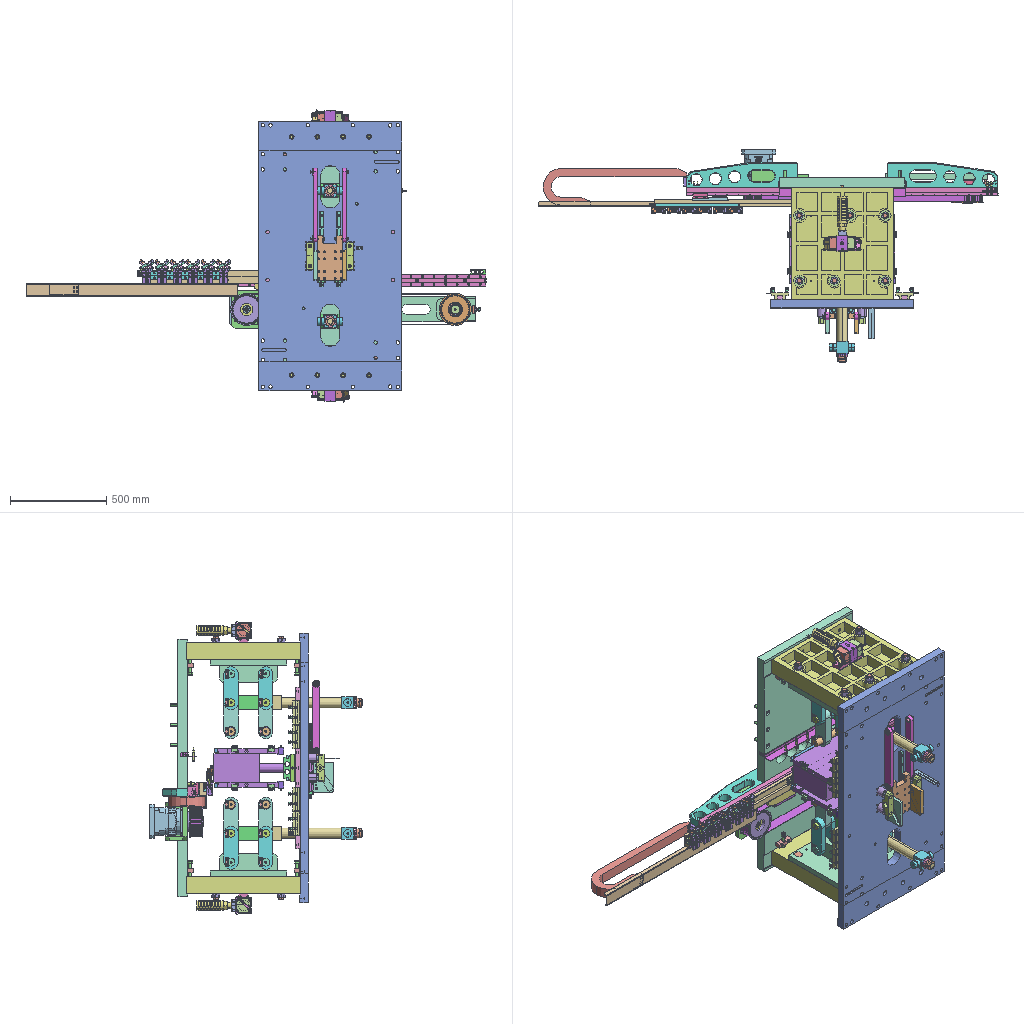Assembly | STEP file | 127 different items | 785 placed | box 2393 x 1108 x 1521 mm
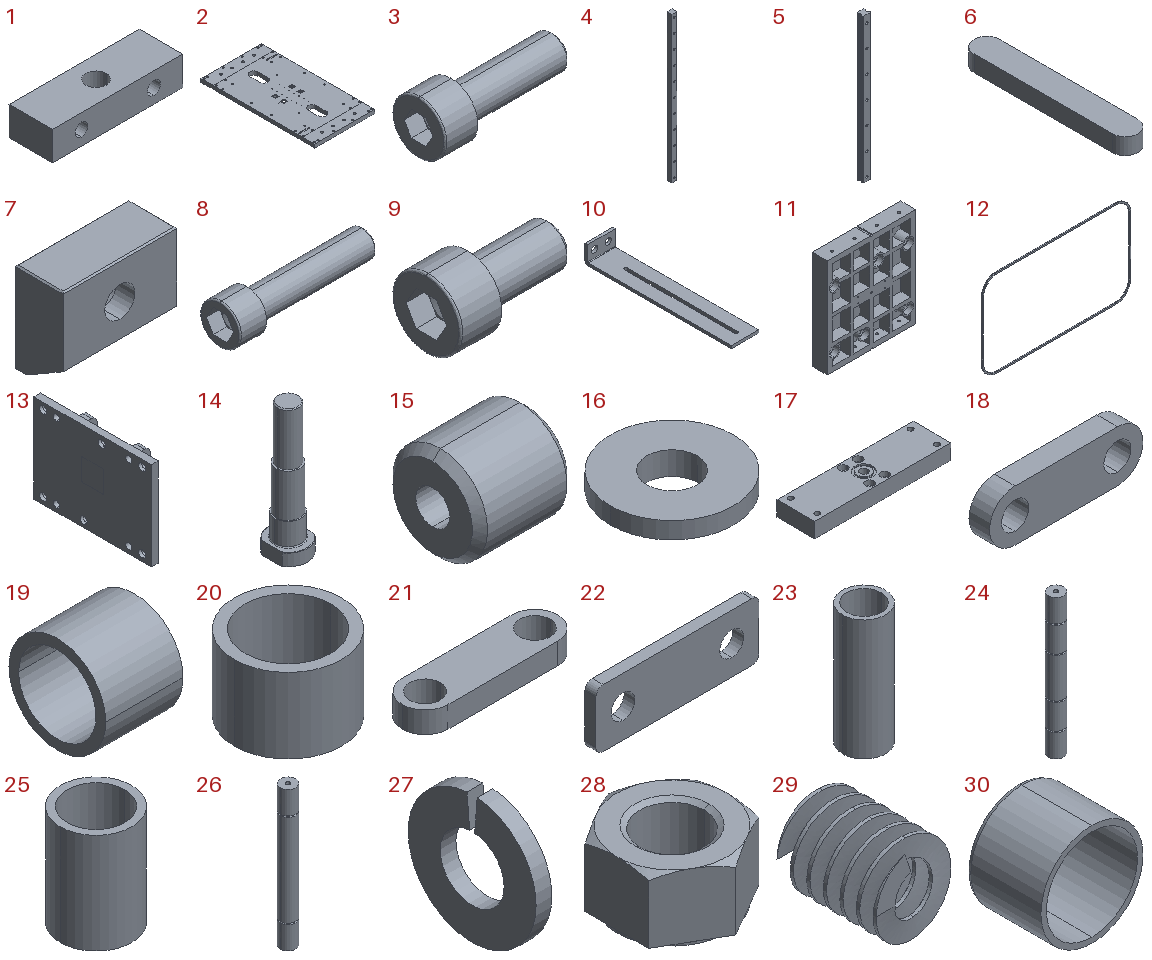Parts list (item | name | quantity | parent item | size | volume):
1 | M-05-2507_default | x8 | in LM06S-05-03-02B_default, LM06S-05-02-04 modified_default | 90 x 30 x 20 mm | 45159 mm3
2 | LM-05-1222B_default | x1 | in LM06S-05-03-02B_default | 742 x 1400 x 44 mm | 38795676 mm3
3 | PN_0075_default | x22 | in LM06S-05-03-02B_default | 33 x 13 x 13 mm | 2167 mm3
4 | P-008160^LM06S-05-03-02B_default | x2 | in LM06S-05-03-02B_default | 28 x 26 x 840 mm | 581403 mm3
5 | P-008244^LM06S-05-03-02B | x2 | in LM06S-05-03-02B_default | 20 x 17.5 x 390 mm | 110981 mm3
6 | PN_0059_default | x4 | in LM06S-05-03-02B_default, LM06S-05-02-04 modified_default | 14 x 90 x 9 mm | 10961 mm3
7 | P-0082091 | x11 | in LM06S-05-03-02B_default | 25 x 10.5 x 20 mm | 3970 mm3
8 | PN_0053_socket head screw-M16x70L | x8 | in LM06S-05-03-02B_default, LM06S-05-02-04 modified_default | 86 x 24 x 24 mm | 19678 mm3
9 | PN_0071_default | x61 | in LM06S-05-03-02B_default, LM06S-05-01-05, LM06S-05-01-06, traverse group | 18 x 10 x 10 mm | 730.412 mm3
10 | LM-05-1060A | x1 | in LM06S-05-03-02B_default | 30 x 160 x 20 mm | 14324 mm3
11 | LM-05-1236 | x2 | in LM06S-05-01-05 | 532 x 90 x 594 mm | 16985002 mm3
12 | P-0102091 | x2 | in LM06S-05-01-05 | 508.6 x 4.6 x 299.7 mm | 33274 mm3
13 | LM-05-1233_default | x2 | in LM06S-05-01-05 | 120 x 532 x 400 mm | 7941008 mm3
14 | LM-05-1234 | x12 | in LM06S-05-01-05 | 37 x 44 x 149.3 mm | 94878 mm3
15 | LM-05-1235_default | x8 | in LM06S-05-01-05 | 25 x 25 x 25 mm | 9411 mm3
16 | LM-05-1133_default | x12 | in LM06S-05-01-05 | 59 x 59 x 11 mm | 18636 mm3
17 | M-05-116C_default | x2 | in LM06S-05-01-05 | 180 x 50 x 20 mm | 168438 mm3
18 | LM-05-1223_default | x16 | in LM06S-05-01-05 | 225 x 30 x 75 mm | 393263 mm3
19 | P-0082107 | x8 | in LM06S-05-01-05 | 40 x 50 x 50 mm | 28274 mm3
20 | LM-05-1226_default | x8 | in LM06S-05-01-05 | 50 x 50 x 35 mm | 24520 mm3
21 | LM-05-1225_default | x4 | in LM06S-05-01-05 | 255 x 75 x 35 mm | 489681 mm3
22 | LM-05-1153A_default | x24 | in LM06S-05-01-05, LM06S-05-01-06 | 45 x 3 x 16 mm | 1944 mm3
23 | LM-05-1229_default | x4 | in LM06S-05-01-05 | 50 x 50 x 140 mm | 98079 mm3
24 | LM-05-1232 | x4 | in LM06S-05-01-05 | 40 x 40 x 361 mm | 429924 mm3
25 | LM-05-1230_default | x2 | in LM06S-05-01-05 | 50 x 50 x 70 mm | 49040 mm3
26 | LM-05-1231 | x4 | in LM06S-05-01-05 | 40 x 40 x 361 mm | 430990 mm3
27 | PN_0038_default | x48 | in LM06S-05-01-05, LM06S-05-01-06 | 1.5 x 12.2 x 12.181 mm | 128.223 mm3
28 | PN_0069_hex nut-M24x3.0 | x24 | in LM06S-05-01-05 | 36 x 41.569 x 21.5 mm | 16438 mm3
29 | PN_0023_default | x12 | in LM06S-05-01-05 | 50 x 60 x 50 mm | 16434 mm3
30 | PN_0016_default | x8 | in LM06S-05-01-05 | 28 x 20 x 28 mm | 2487 mm3
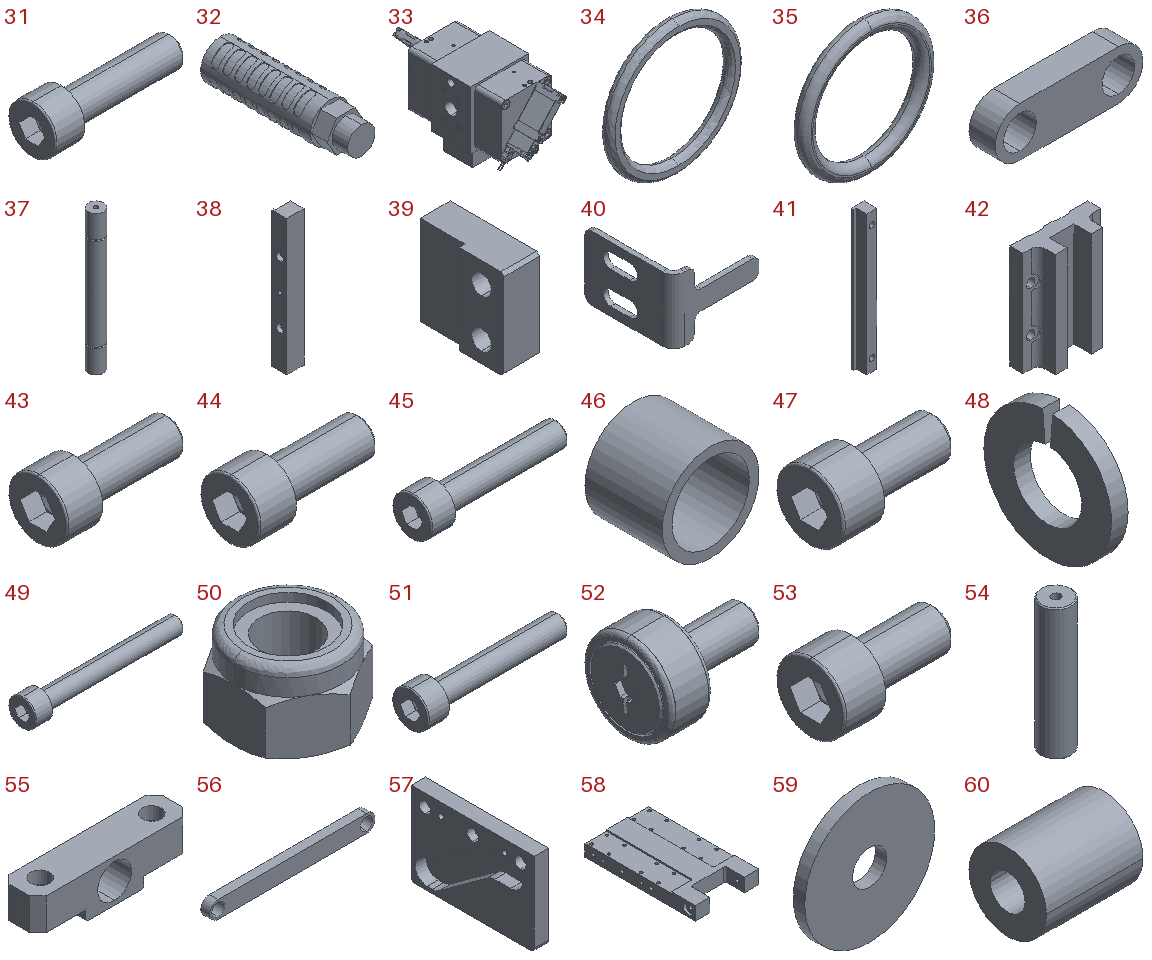31 | PN_0043_default | x16 | in LM06S-05-01-05, LM06S-05-02-04 modified_default | 38 x 13 x 13 mm | 2418 mm3
32 | PN_0013_default | x2 | in LM06S-05-01-05 | 50 x 180 x 50 mm | 314357 mm3
33 | PN_0049_default | x2 | in LM06S-05-01-05 | 91.232 x 195.93 x 105 mm | 684880 mm3
34 | PN_0034_default | x2 | in LM06S-05-01-05 | 24.8 x 2.3 x 24.8 mm | 313.815 mm3
35 | PN_0002_default | x2 | in LM06S-05-01-05 | 31.7 x 3.49 x 31.7 mm | 852.143 mm3
36 | LM-05-1240_default | x8 | in LM06S-05-01-06 | 225 x 40 x 75 mm | 469635 mm3
37 | LM-05-1241 | x4 | in LM06S-05-01-06 | 40 x 40 x 361 mm | 430990 mm3
38 | LM-05-1243_default | x4 | in LM06S-05-01-06 | 35 x 30 x 274 mm | 250341 mm3
39 | M-05-006A_default | x8 | in LM06S-05-01-06 | 12 x 30 x 30 mm | 8337 mm3
40 | M-05-748A_default | x2 | in LM06S-05-01-06 | 26.5 x 27.5 x 20 mm | 981.783 mm3
41 | LM-05-1197_default | x4 | in LM06S-05-01-06 | 21 x 21 x 230 mm | 79008 mm3
42 | P-008108 | x8 | in LM06S-05-01-06 | 90 x 36 x 120.4 mm | 224180 mm3
43 | PN_0066_default | x16 | in LM06S-05-01-06 | 22 x 10 x 10 mm | 844.002 mm3
44 | PN_0009_default | x32 | in LM06S-05-01-06 | 35 x 16 x 16 mm | 3637 mm3
45 | PN_0007_default | x8 | in LM06S-05-01-06 | 48 x 13 x 13 mm | 2921 mm3
46 | P-0082107^LM06S-05-01-06 | x16 | in LM06S-05-01-06 | 50 x 40 x 50 mm | 28274 mm3
47 | PN_0040_default | x2 | in LM06S-05-06B | 24 x 13 x 13 mm | 1714 mm3
48 | PN_0025_default | x4 | in LM06S-05-06B | 2 x 15.4 x 15.376 mm | 260.237 mm3
49 | PN_0029_default | x2 | in LM06S-05-06B | 73 x 13 x 13 mm | 4180 mm3
50 | P-006032 | x2 | in LM06S-05-06B | 13 x 15.011 x 9.5 mm | 952.721 mm3
51 | PN_0056_socket head screw-M5x35 | x16 | in LM06S-05-06B | 35 x 8.5 x 8.5 mm | 829.835 mm3
52 | PN_0073_default | x2 | in LM06S-05-06B | 40 x 30 x 30 mm | 12542 mm3
53 | PN_0018_default | x16 | in LM06S-05-06B | 18 x 10 x 10 mm | 730.412 mm3
54 | LM-05-1254B_default | x4 | in LM06S-05-06B | 30 x 30 x 130.5 mm | 89786 mm3
55 | LM-05-1255B_default | x2 | in LM06S-05-06B | 145 x 35 x 40 mm | 134466 mm3
56 | LM-05-1256_default | x2 | in LM06S-05-06B | 387.07 x 20 x 40 mm | 274514 mm3
57 | LM-05-1257B | x1 | in LM06S-05-06B | 18 x 155 x 105 mm | 225163 mm3
58 | LM-05-1260 | x1 | in LM06S-05-06B | 132 x 230 x 28 mm | 697857 mm3
59 | LM-05-1261B | x4 | in LM06S-05-06B | 34 x 3 x 34 mm | 2533 mm3
60 | LM-05-1262 | x2 | in LM06S-05-06B | 25 x 20 x 20 mm | 6264 mm3
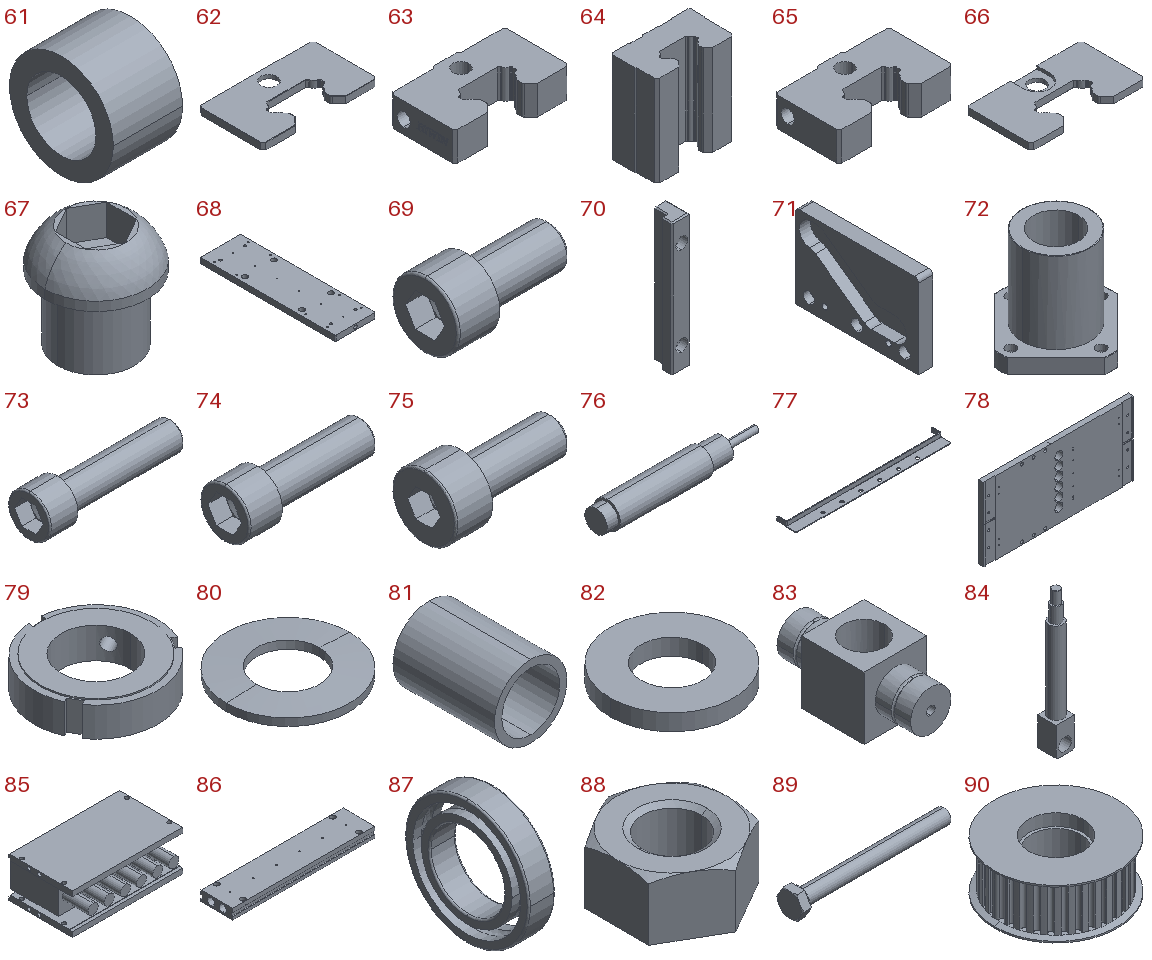61 | P-008247^LM06S-05-06B | x4 | in LM06S-05-06B | 20 x 30 x 30 mm | 7854 mm3
62 | PART1AAA^SUB1AA_P-008243 | x4 | in SUB1AA^P-008243 | 43 x 24.4 x 2.5 mm | 1956 mm3
63 | PART2A^SUB1AA_P-008243 | x4 | in SUB1AA^P-008243 | 43 x 25.2 x 11 mm | 8694 mm3
64 | PART3A^SUB1AA_P-008243 | x4 | in SUB1AA^P-008243 | 44 x 25.4 x 50.5 mm | 44203 mm3
65 | PART4^SUB1AA_P-008243 | x4 | in SUB1AA^P-008243 | 43 x 25.2 x 11 mm | 8694 mm3
66 | PART5A^SUB1AA_P-008243 | x4 | in SUB1AA^P-008243 | 43 x 24.4 x 2.5 mm | 1956 mm3
67 | M6H^P-008243 | x4 | in P-008243 | 8 x 8 x 8 mm | 227.362 mm3
68 | LM-05-1224B_default | x1 | in LM06S-05-06B | 145 x 490 x 20 mm | 1346383 mm3
69 | PN_0067_socket head screw-M10x20L | x4 | in LM06S-05-06B | 30 x 16 x 16 mm | 3244 mm3
70 | LM-05-1228 | x4 | in LM06S-05-06B | 15.5 x 20 x 120 mm | 29201 mm3
71 | LM-05-1258B | x1 | in LM06S-05-06B | 18 x 155 x 105 mm | 224873 mm3
72 | PN_0010_default | x4 | in LM06S-05-06B | 74 x 74 x 64 mm | 70760 mm3
73 | P-001093_JIS B 1176 M16 x 50 (50) --N | x6 | in LM06S-05-02-04 modified_default | 81 x 24 x 24 mm | 18678 mm3
74 | P-001072_JIS B 1176 M16 x 50 (50) --N | x8 | in LM06S-05-02-04 modified_default | 66 x 24 x 24 mm | 15657 mm3
75 | PN_0028_default | x4 | in LM06S-05-02-04 modified_default | 14 x 7 x 7 mm | 260.117 mm3
76 | PN_0014_default | x10 | in LM06S-05-02-04 modified_default, traverse group | 72 x 12 x 12 mm | 6034 mm3
77 | LM-05-1212_default | x1 | in LM06S-05-02-04 modified_default | 656 x 82 x 20 mm | 121048 mm3
78 | forming top plate | x1 | in LM06S-05-02-04 modified_default | 1340 x 50 x 650 mm | 41398867 mm3
79 | PN_0019_default | x4 | in LM06S-05-04-02 | 48 x 47.869 x 12 mm | 14121 mm3
80 | PN_0065_default | x4 | in LM06S-05-04-02 | 60 x 60 x 4.5 mm | 7770 mm3
81 | PN_0036_default | x2 | in LM06S-05-04-02 | 50 x 70 x 50 mm | 49480 mm3
82 | LM-05-1237_default | x2 | in LM06S-05-04-02 | 60 x 60 x 8 mm | 16889 mm3
83 | LM-05-1238 | x2 | in LM06S-05-04-02 | 62 x 132 x 62 mm | 244471 mm3
84 | LM-05-1239_default | x2 | in LM06S-05-04-02 | 70 x 70 x 538 mm | 1281973 mm3
85 | mold 06_default | x1 | in PN_0012 mold_default | 545 x 363.5 x 200 mm | 24295662 mm3
86 | LM-05-1227_default | x1 | in PN_0012 mold_default | 490 x 110 x 35 mm | 1412301 mm3
87 | PN_0027_default | x2 | in LM06S-05-02-02 modified_default | 16 x 75 x 75 mm | 27632 mm3
88 | PN_0064_hex nut-M12x1.75 | x3 | in LM06S-05-02-02 modified_default | 19 x 21.939 x 10 mm | 2282 mm3
89 | PN_0001_hex bolt-M10x55L | x1 | in LM06S-05-02-02 modified_default | 106.4 x 18.475 x 16 mm | 9247 mm3
90 | LM-05-1157 modified_default | x1 | in LM06S-05-02-02 modified_default | 168 x 168 x 68 mm | 926105 mm3
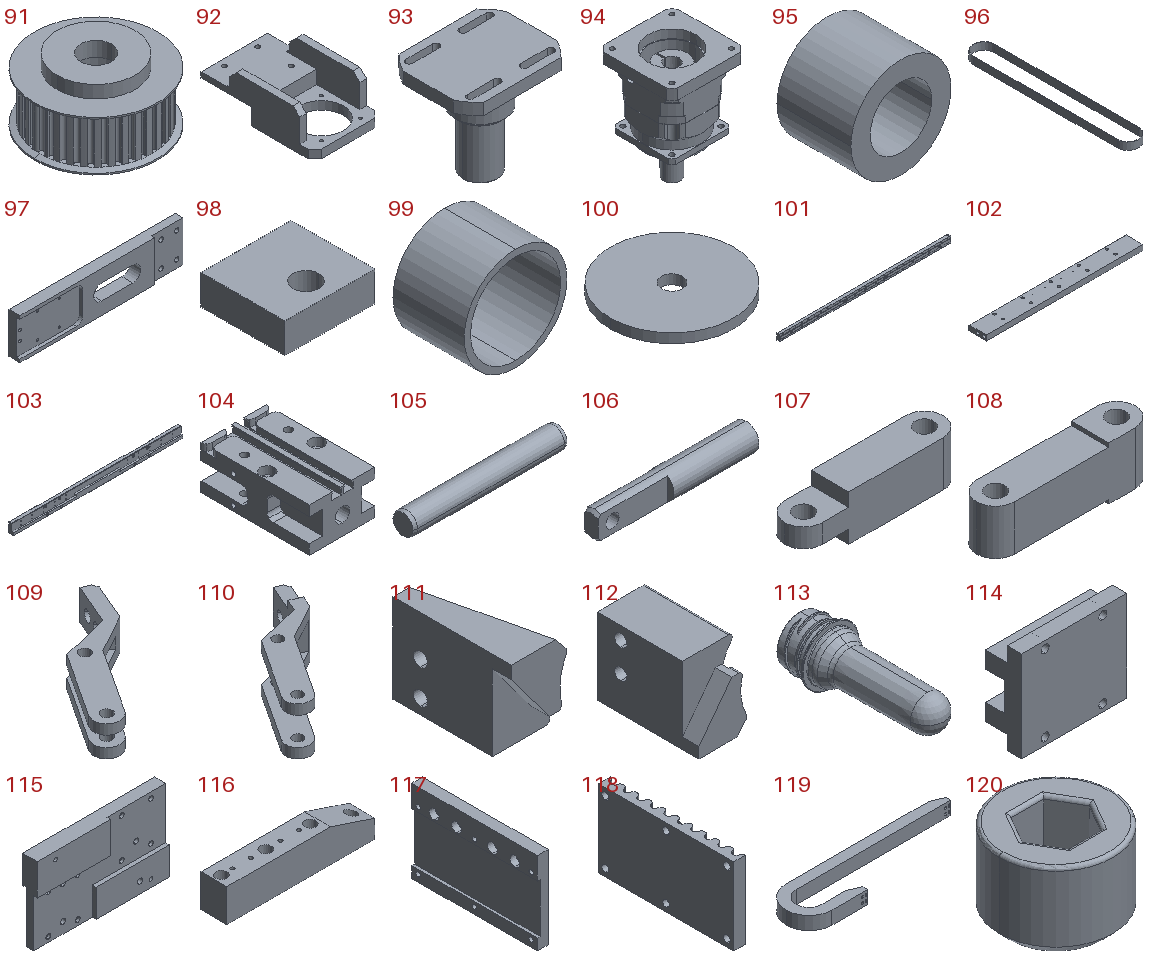91 | LM-05-1158_default | x1 | in LM06S-05-02-02 modified_default | 168 x 168 x 85 mm | 1104841 mm3
92 | LM-05-1159_default | x1 | in LM06S-05-02-02 modified_default | 200 x 340 x 115 mm | 1813258 mm3
93 | LM-05-1162 modified_default | x1 | in LM06S-05-02-02 modified_default | 135 x 110 x 129 mm | 443950 mm3
94 | PN_0046_default | x1 | in LM06S-05-02-02 modified_default | 176 x 176 x 263.5 mm | 3077737 mm3
95 | PN_0061_default | x1 | in LM06S-05-02-02 modified_default | 65 x 48 x 65 mm | 98960 mm3
96 | timing belt 14M-2660L_default | x1 | in LM06S-05-02-02 modified_default | 161.176 x 1246 x 55 mm | 381989 mm3
97 | fixing plate_default | x1 | in LM06S-05-02-02 modified_default | 530 x 35 x 130 mm | 1787786 mm3
98 | adjusting block_default | x1 | in LM06S-05-02-02 modified_default | 45 x 42 x 15 mm | 24875 mm3
99 | bearing spacer_default | x1 | in LM06S-05-02-02 modified_default | 52 x 36 x 52 mm | 17919 mm3
100 | limit plate_default | x1 | in LM06S-05-02-02 modified_default | 52 x 52 x 4 mm | 8240 mm3
101 | rail fixing plate | x1 | in traverse group | 1620 x 30 x 60 mm | 2595354 mm3
102 | LM-05-1206 modified_default | x2 | in traverse group | 445 x 50 x 15 mm | 275909 mm3
103 | traverse rod | x1 | in traverse group | 1200 x 35 x 70 mm | 2126104 mm3
104 | PN_0068^seat_default | x12 | in seat_default | 45 x 74.5 x 30 mm | 67519 mm3
105 | - | x24 | in seat_default | 35 x 5 x 5 mm | 684.607 mm3
106 | mandrel_default | x12 | in gripper cylinder_closed, gripper cylinder_open | 59 x 10 x 10 mm | 3717 mm3
107 | gripper arm 1_default | x12 | in gripper cylinder_closed, gripper cylinder_open | 42 x 10 x 12 mm | 3684 mm3
108 | gripper arm 2_default | x12 | in gripper cylinder_closed, gripper cylinder_open | 42 x 10 x 14 mm | 4491 mm3
109 | gripper arm 4_default | x12 | in gripper cylinder_closed, gripper cylinder_open | 54.647 x 62.275 x 14 mm | 6777 mm3
110 | gripper arm 3_default | x12 | in gripper cylinder_closed, gripper cylinder_open | 54.647 x 62.275 x 24 mm | 7898 mm3
111 | CLM-5001A | x12 | in gripper cylinder_closed, gripper cylinder_open | 13.626 x 28 x 21 mm | 5621 mm3
112 | CLM-5002A | x12 | in gripper cylinder_closed, gripper cylinder_open | 13.626 x 28 x 21 mm | 5621 mm3
113 | 30-25 bottle preform_default | x6 | in gripper cylinder_closed | 34 x 86.5 x 34 mm | 12147 mm3
114 | copy of MSA20EA.stp^PN_0017_default | x4 | in PN_0017_default | 72.9 x 25 x 63 mm | 72025 mm3
115 | slider fixing plate | x2 | in traverse group | 180 x 20 x 108 mm | 259977 mm3
116 | connecting block | x1 | in traverse group | 200 x 35 x 44.5 mm | 266252 mm3
117 | LM-05-1163 modified_default | x1 | in traverse group | 12 x 140 x 92 mm | 126847 mm3
118 | LM-05-1155 modified_default | x1 | in traverse group | 12 x 140 x 80 mm | 99342 mm3
119 | P-0171514 modified_default | x1 | in traverse group | 746 x 192 x 55 mm | 1359161 mm3
120 | P-015007 | x4 | in traverse group | 9.8 x 9.8 x 7 mm | 415.303 mm3
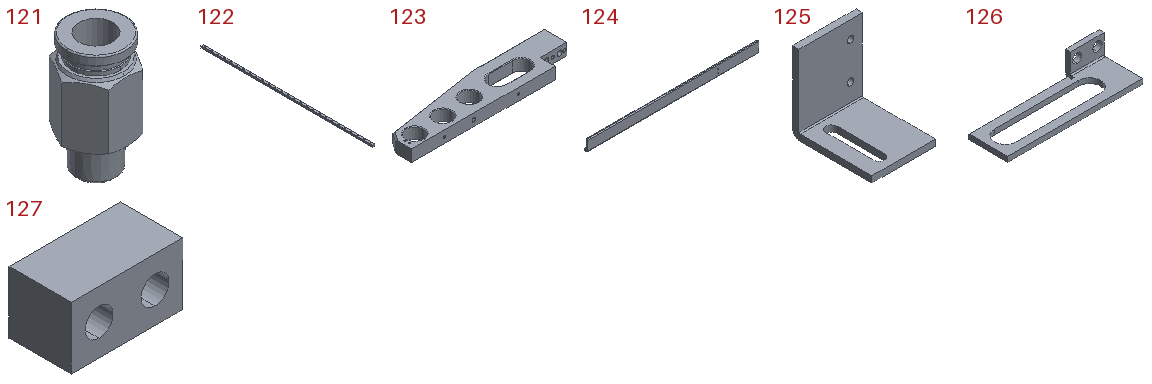121 | PN_0022_default | x4 | in traverse group | 16.166 x 14 x 27.9 mm | 2758 mm3
122 | P-0082097 modified_default | x2 | in traverse group | 20 x 1620 x 18 mm | 560839 mm3
123 | reinforcing fixing bracket | x2 | in traverse group | 575 x 130 x 40 mm | 1733359 mm3
124 | drag chain fixing plate_default | x1 | in traverse group | 1100 x 25 x 68 mm | 406508 mm3
125 | drag chain fixing sheet metal_default | x1 | in traverse group | 40 x 50 x 50 mm | 14067 mm3
126 | detection sheet metal_default | x2 | in traverse group | 80 x 26 x 15 mm | 3862 mm3
127 | limit block | x2 | in traverse group | 18 x 10 x 10 mm | 1180 mm3
Placements (level | parent | child | x y z in mm | rotation matrix by rows), first 229 of 833 lines:
1 | mold base | LM06S-05-03-02B_default | 0.0 184.089 0.0 | 1 0 0 0 0 1 0 -1 -0
2 | LM06S-05-03-02B_default | M-05-2507_default | 135.477 85.671 -140.089 | -1 0 0 0 0 1 0 1 0
2 | LM06S-05-03-02B_default | M-05-2507_default | 135.477 1155.671 -140.089 | -1 0 0 0 0 1 0 1 0
2 | LM06S-05-03-02B_default | M-05-2507_default | 377.478 105.671 -140.089 | 1 0 0 0 0 -1 0 1 -0
2 | LM06S-05-03-02B_default | M-05-2507_default | 377.478 1175.671 -140.089 | 1 0 0 0 0 -1 0 1 -0
2 | LM06S-05-03-02B_default | LM-05-1222B_default | -380.522 605.672 -162.089 | -1 0 0 0 1 0 0 0 -1
2 | LM06S-05-03-02B_default | PN_0075_default | 580.477 1030.671 -123.089 | 0 0.8924 0.4513 0 0.4513 -0.8924 -1 0 -0
2 | LM06S-05-03-02B_default | PN_0075_default | 580.477 230.672 -123.089 | 0 0.8924 0.4513 0 0.4513 -0.8924 -1 0 -0
2 | LM06S-05-03-02B_default | PN_0075_default | 580.477 310.671 -123.089 | 0 0.8924 0.4513 0 0.4513 -0.8924 -1 0 -0
2 | LM06S-05-03-02B_default | PN_0075_default | 580.477 390.671 -123.089 | 0 0.8924 0.4513 0 0.4513 -0.8924 -1 0 -0
2 | LM06S-05-03-02B_default | PN_0075_default | 580.477 470.671 -123.089 | 0 0.8924 0.4513 0 0.4513 -0.8924 -1 0 -0
2 | LM06S-05-03-02B_default | PN_0075_default | 580.477 550.672 -123.089 | 0 0.8924 0.4513 0 0.4513 -0.8924 -1 0 -0
2 | LM06S-05-03-02B_default | PN_0075_default | 580.477 630.672 -123.089 | 0 0.8924 0.4513 0 0.4513 -0.8924 -1 0 -0
2 | LM06S-05-03-02B_default | PN_0075_default | 580.477 710.672 -123.089 | 0 0.8924 0.4513 0 0.4513 -0.8924 -1 0 -0
2 | LM06S-05-03-02B_default | PN_0075_default | 580.477 790.672 -123.089 | 0 0.8924 0.4513 0 0.4513 -0.8924 -1 0 -0
2 | LM06S-05-03-02B_default | PN_0075_default | 580.477 870.672 -123.089 | 0 0.8924 0.4513 0 0.4513 -0.8924 -1 0 -0
2 | LM06S-05-03-02B_default | PN_0075_default | 580.477 950.672 -123.089 | 0 0.8924 0.4513 0 0.4513 -0.8924 -1 0 -0
2 | LM06S-05-03-02B_default | PN_0075_default | -67.522 1030.671 -123.089 | 0 -0.4605 0.8877 0 0.8877 0.4605 -1 0 -0
2 | LM06S-05-03-02B_default | PN_0075_default | -67.522 230.672 -123.089 | 0 -0.4605 0.8877 0 0.8877 0.4605 -1 0 -0
2 | LM06S-05-03-02B_default | PN_0075_default | -67.522 310.671 -123.089 | 0 -0.4605 0.8877 0 0.8877 0.4605 -1 0 -0
2 | LM06S-05-03-02B_default | PN_0075_default | -67.522 390.671 -123.089 | 0 -0.4605 0.8877 0 0.8877 0.4605 -1 0 -0
2 | LM06S-05-03-02B_default | PN_0075_default | -67.522 470.671 -123.089 | 0 -0.4605 0.8877 0 0.8877 0.4605 -1 0 -0
2 | LM06S-05-03-02B_default | PN_0075_default | -67.522 550.672 -123.089 | 0 -0.4605 0.8877 0 0.8877 0.4605 -1 0 -0
2 | LM06S-05-03-02B_default | PN_0075_default | -67.522 630.672 -123.089 | 0 -0.4605 0.8877 0 0.8877 0.4605 -1 0 -0
2 | LM06S-05-03-02B_default | PN_0075_default | -67.522 710.672 -123.089 | 0 -0.4605 0.8877 0 0.8877 0.4605 -1 0 -0
2 | LM06S-05-03-02B_default | PN_0075_default | -67.522 790.672 -123.089 | 0 -0.4605 0.8877 0 0.8877 0.4605 -1 0 -0
2 | LM06S-05-03-02B_default | PN_0075_default | -67.522 870.672 -123.089 | 0 -0.4605 0.8877 0 0.8877 0.4605 -1 0 -0
2 | LM06S-05-03-02B_default | PN_0075_default | -67.522 950.672 -123.089 | 0 -0.4605 0.8877 0 0.8877 0.4605 -1 0 -0
2 | LM06S-05-03-02B_default | P-008160^LM06S-05-03-02B_default | 566.477 1050.671 -145.089 | 1 0 0 0 0 -1 0 1 -0
2 | LM06S-05-03-02B_default | P-008160^LM06S-05-03-02B_default | -81.522 1050.671 -145.089 | 1 0 0 0 0 -1 0 1 -0
2 | LM06S-05-03-02B_default | P-008244^LM06S-05-03-02B | 300.478 290.671 -184.089 | -1 0 0 0 0 -1 0 -1 0
2 | LM06S-05-03-02B_default | P-008244^LM06S-05-03-02B | 212.477 290.671 -184.089 | -1 0 0 0 0 -1 0 -1 0
2 | LM06S-05-03-02B_default | PN_0059_default | 256.478 1240.671 -144.589 | 1 0 0 0 1 0 0 0 1
2 | LM06S-05-03-02B_default | PN_0059_default | 256.478 20.672 -144.589 | 1 0 0 0 1 0 0 0 1
2 | LM06S-05-03-02B_default | P-0082091 | 604.477 1030.679 -145.944 | 0.003842 0 -1 -1 0 -0.003842 0 1 -0
2 | LM06S-05-03-02B_default | P-0082091 | 604.477 230.679 -145.944 | 0.003842 0 -1 -1 0 -0.003842 0 1 -0
2 | LM06S-05-03-02B_default | P-0082091 | 604.477 310.679 -145.944 | 0.003842 0 -1 -1 0 -0.003842 0 1 -0
2 | LM06S-05-03-02B_default | P-0082091 | 604.477 390.679 -145.944 | 0.003842 0 -1 -1 0 -0.003842 0 1 -0
2 | LM06S-05-03-02B_default | P-0082091 | 604.477 470.679 -145.944 | 0.003842 0 -1 -1 0 -0.003842 0 1 -0
2 | LM06S-05-03-02B_default | P-0082091 | 604.477 550.679 -145.944 | 0.003842 0 -1 -1 0 -0.003842 0 1 -0
2 | LM06S-05-03-02B_default | P-0082091 | 604.477 630.679 -145.944 | 0.003842 0 -1 -1 0 -0.003842 0 1 -0
2 | LM06S-05-03-02B_default | P-0082091 | 604.477 710.679 -145.944 | 0.003842 0 -1 -1 0 -0.003842 0 1 -0
2 | LM06S-05-03-02B_default | P-0082091 | 604.477 790.679 -145.944 | 0.003842 0 -1 -1 0 -0.003842 0 1 -0
2 | LM06S-05-03-02B_default | P-0082091 | 604.477 870.679 -145.944 | 0.003842 0 -1 -1 0 -0.003842 0 1 -0
2 | LM06S-05-03-02B_default | P-0082091 | 604.477 950.679 -145.944 | 0.003842 0 -1 -1 0 -0.003842 0 1 -0
2 | LM06S-05-03-02B_default | PN_0053_socket head screw-M16x70L | 90.478 151.672 -125.089 | 0 -0.7841 0.6206 -1 0 0 0 -0.6206 -0.7841
2 | LM06S-05-03-02B_default | PN_0053_socket head screw-M16x70L | 422.478 151.672 -125.089 | 0 0.7841 0.6206 -1 0 0 0 -0.6206 0.7841
2 | LM06S-05-03-02B_default | PN_0053_socket head screw-M16x70L | 90.478 1109.671 -125.089 | 0 -0.7841 -0.6206 1 0 0 0 -0.6206 0.7841
2 | LM06S-05-03-02B_default | PN_0053_socket head screw-M16x70L | 422.478 1109.671 -125.089 | 0 0.7841 -0.6206 1 0 0 0 -0.6206 -0.7841
2 | LM06S-05-03-02B_default | PN_0071_default | 602.477 1030.671 -140.694 | 0 -0.5188 0.8549 0 0.8549 0.5188 -1 0 0
2 | LM06S-05-03-02B_default | PN_0071_default | 602.477 230.672 -140.694 | 0 -0.5188 0.8549 0 0.8549 0.5188 -1 0 0
2 | LM06S-05-03-02B_default | PN_0071_default | 602.477 310.671 -140.694 | 0 -0.5188 0.8549 0 0.8549 0.5188 -1 0 0
2 | LM06S-05-03-02B_default | PN_0071_default | 602.477 390.671 -140.694 | 0 -0.5188 0.8549 0 0.8549 0.5188 -1 0 0
2 | LM06S-05-03-02B_default | PN_0071_default | 602.477 470.671 -140.694 | 0 -0.5188 0.8549 0 0.8549 0.5188 -1 0 0
2 | LM06S-05-03-02B_default | PN_0071_default | 602.477 550.672 -140.694 | 0 -0.5188 0.8549 0 0.8549 0.5188 -1 0 0
2 | LM06S-05-03-02B_default | PN_0071_default | 602.477 630.672 -140.694 | 0 -0.5188 0.8549 0 0.8549 0.5188 -1 0 0
2 | LM06S-05-03-02B_default | PN_0071_default | 602.477 710.672 -140.694 | 0 -0.5188 0.8549 0 0.8549 0.5188 -1 0 0
2 | LM06S-05-03-02B_default | PN_0071_default | 602.477 790.672 -140.694 | 0 -0.5188 0.8549 0 0.8549 0.5188 -1 0 0
2 | LM06S-05-03-02B_default | PN_0071_default | 602.477 870.672 -140.694 | 0 -0.5188 0.8549 0 0.8549 0.5188 -1 0 0
2 | LM06S-05-03-02B_default | PN_0071_default | 602.477 950.672 -140.694 | 0 -0.5188 0.8549 0 0.8549 0.5188 -1 0 0
2 | LM06S-05-03-02B_default | LM-05-1060A | 407.978 581.672 -264.089 | -1 0 0 0 0 1 0 1 -0
1 | mold base | LM06S-05-01-05 | -83.166 -156.734 -184.107 | 1 0 0 0 0 1 0 -1 0
2 | LM06S-05-01-05 | LM-05-1236 | 339.644 -134.31 519.734 | 1 0 0 0 1 0 0 0 1
2 | LM06S-05-01-05 | P-0102091 | 334.144 -115.585 473.234 | 1 0 0 0 -1 0 0 0 -1
2 | LM06S-05-01-05 | LM-05-1233_default | 339.644 -103.435 417.734 | 0 -1 0 1 0 0 0 0 1
2 | LM06S-05-01-05 | LM-05-1234 | 563.144 -88.935 637.734 | 1 0 0 0 0 -1 0 1 0
2 | LM06S-05-01-05 | LM-05-1234 | 380.644 -88.935 637.734 | 1 0 0 0 0 -1 0 1 0
2 | LM06S-05-01-05 | LM-05-1234 | 116.144 -88.935 637.734 | 1 0 0 0 0 -1 0 1 0
2 | LM06S-05-01-05 | LM-05-1234 | 563.144 -88.935 297.734 | 1 0 0 0 0 -1 0 1 0
2 | LM06S-05-01-05 | LM-05-1234 | 116.144 -88.935 297.734 | 1 0 0 0 0 -1 0 1 0
2 | LM06S-05-01-05 | LM-05-1234 | 298.644 -88.935 297.734 | 1 0 0 0 0 -1 0 1 0
2 | LM06S-05-01-05 | LM-05-1235_default | 503.144 -113.435 637.734 | 0 -0.9752 -0.2214 1 0 0 0 -0.2214 0.9752
2 | LM06S-05-01-05 | LM-05-1235_default | 176.144 -113.435 297.734 | 0 0.3995 -0.9167 1 0 0 0 -0.9167 -0.3995
2 | LM06S-05-01-05 | LM-05-1235_default | 503.144 -113.435 297.734 | 0 0.3995 -0.9167 1 0 0 0 -0.9167 -0.3995
2 | LM06S-05-01-05 | LM-05-1235_default | 176.144 -113.435 637.734 | 0 0.3995 -0.9167 1 0 0 0 -0.9167 -0.3995
2 | LM06S-05-01-05 | LM-05-1133_default | 563.144 -180.435 637.734 | 0.9816 0.191 0 0 0 -1 -0.191 0.9816 0
2 | LM06S-05-01-05 | LM-05-1133_default | 116.144 -180.435 637.734 | 0.9816 0.191 0 0 0 -1 -0.191 0.9816 0
2 | LM06S-05-01-05 | LM-05-1133_default | 298.644 -180.435 297.734 | 0.9814 0.1919 0 0 0 -1 -0.1919 0.9814 0
2 | LM06S-05-01-05 | LM-05-1133_default | 116.144 -180.435 297.734 | 0.9814 0.1919 0 0 0 -1 -0.1919 0.9814 0
2 | LM06S-05-01-05 | LM-05-1133_default | 563.144 -180.435 297.734 | 0.9816 0.191 0 0 0 -1 -0.191 0.9816 0
2 | LM06S-05-01-05 | LM-05-1133_default | 380.644 -180.435 637.734 | 0.9816 0.191 0 0 0 -1 -0.191 0.9816 0
2 | LM06S-05-01-05 | M-05-116C_default | 339.644 -228.435 492.734 | -1 0 0 0 0 1 0 1 -0
2 | LM06S-05-01-05 | LM-05-1223_default | 424.644 39.56 367.734 | 0 1 0 -1 0 0 0 0 1
2 | LM06S-05-01-05 | LM-05-1223_default | 324.644 23.57 367.734 | 0 -1 0 1 0 0 0 0 1
2 | LM06S-05-01-05 | P-0082107 | 469.644 -43.435 377.734 | 1 0 0 0 -0.6534 -0.757 0 0.757 -0.6534
2 | LM06S-05-01-05 | P-0082107 | 229.644 -43.435 557.734 | 1 0 0 0 0.5086 0.861 0 -0.861 0.5086
2 | LM06S-05-01-05 | P-0082107 | 469.644 -43.435 557.734 | 1 0 0 0 0.8649 0.502 0 -0.502 0.8649
2 | LM06S-05-01-05 | LM-05-1223_default | 324.644 23.57 547.734 | 0 -1 0 1 0 0 0 0 1
2 | LM06S-05-01-05 | P-0082107 | 229.644 -43.435 377.734 | 1 0 0 0 0.9486 0.3164 0 -0.3164 0.9486
2 | LM06S-05-01-05 | LM-05-1226_default | 392.144 106.565 557.734 | 0 0 1 -0.8192 0.5736 0 -0.5736 -0.8192 0
2 | LM06S-05-01-05 | LM-05-1226_default | 287.144 106.565 557.734 | 0 0 -1 0.8192 -0.5736 0 -0.5736 -0.8192 -0
2 | LM06S-05-01-05 | LM-05-1225_default | 287.144 106.565 467.734 | 0 0 1 0 -1 0 1 0 0
2 | LM06S-05-01-05 | LM-05-1223_default | 254.644 23.57 547.734 | 0 -1 0 1 0 0 0 0 1
2 | LM06S-05-01-05 | LM-05-1223_default | 424.644 39.56 547.734 | 0 1 0 -1 0 0 0 0 1
2 | LM06S-05-01-05 | LM-05-1225_default | 392.144 106.565 467.734 | 0 0 -1 0 -1 0 -1 0 -0
2 | LM06S-05-01-05 | LM-05-1223_default | 354.644 39.56 367.734 | 0 1 0 -1 0 0 0 0 1
2 | LM06S-05-01-05 | LM-05-1223_default | 354.644 39.56 547.734 | 0 1 0 -1 0 0 0 0 1
2 | LM06S-05-01-05 | LM-05-1223_default | 254.644 23.57 367.734 | 0 -1 0 1 0 0 0 0 1
2 | LM06S-05-01-05 | LM-05-1153A_default | 168.144 106.565 400.734 | 0 -1 0 -1 0 0 0 0 -1
2 | LM06S-05-01-05 | LM-05-1153A_default | 168.144 106.565 580.734 | 0 -1 0 -1 0 0 0 0 -1
2 | LM06S-05-01-05 | LM-05-1153A_default | 168.144 -43.383 399.486 | 0 -1 0 -0.9965 0 0.08326 -0.08326 0 -0.9965
2 | LM06S-05-01-05 | LM-05-1153A_default | 168.144 -43.435 580.734 | 0 -1 0 -1 0 0 0 0 -1
2 | LM06S-05-01-05 | LM-05-1153A_default | 511.144 106.565 580.734 | 0 1 0 -1 0 0 0 0 1
2 | LM06S-05-01-05 | LM-05-1153A_default | 511.144 106.565 400.734 | 0 1 0 -1 0 0 0 0 1
2 | LM06S-05-01-05 | LM-05-1153A_default | 511.144 -43.435 400.734 | 0 1 0 -1 0 0 0 0 1
2 | LM06S-05-01-05 | LM-05-1153A_default | 511.144 -43.435 580.734 | 0 1 0 -1 0 0 0 0 1
2 | LM06S-05-01-05 | LM-05-1229_default | 339.644 -43.435 377.734 | 0 0 1 0.006481 1 0 -1 0.006481 0
2 | LM06S-05-01-05 | LM-05-1232 | 339.644 106.565 377.734 | 0 0 1 1 0 0 0 1 0
2 | LM06S-05-01-05 | LM-05-1230_default | 339.644 106.565 557.734 | 0 0 1 0.8418 -0.5398 0 0.5398 0.8418 0
2 | LM06S-05-01-05 | LM-05-1231 | 339.644 -43.435 557.734 | 0 0 1 1 0 0 0 1 0
2 | LM06S-05-01-05 | LM-05-1229_default | 339.644 -43.435 557.734 | 0 0 1 0.9701 -0.2426 0 0.2426 0.9701 0
2 | LM06S-05-01-05 | LM-05-1226_default | 287.144 106.565 377.734 | 0 0 -1 0.8192 -0.5736 0 -0.5736 -0.8192 -0
2 | LM06S-05-01-05 | LM-05-1231 | 339.644 -43.435 377.734 | 0 0 1 1 0 0 0 1 0
2 | LM06S-05-01-05 | LM-05-1226_default | 392.144 106.565 377.734 | 0 0 1 -0.8192 0.5736 0 -0.5736 -0.8192 0
2 | LM06S-05-01-05 | LM-05-1232 | 339.644 106.565 557.734 | 0 0 -1 -1 0 0 0 1 -0
2 | LM06S-05-01-05 | PN_0071_default | 159.144 121.565 400.734 | 1 0 0 0 -0.9529 -0.3032 0 0.3032 -0.9529
2 | LM06S-05-01-05 | PN_0071_default | 159.144 -58.435 580.734 | 1 0 0 0 -0.8814 -0.4723 0 0.4723 -0.8814
2 | LM06S-05-01-05 | PN_0038_default | 166.644 -28.435 580.734 | 1 0 0 0 -0.7635 0.6458 0 -0.6458 -0.7635
2 | LM06S-05-01-05 | PN_0071_default | 159.144 -28.435 580.734 | 1 0 0 0 -0.9529 -0.3032 0 0.3032 -0.9529
2 | LM06S-05-01-05 | PN_0071_default | 159.144 -28.435 400.734 | 1 0 0 0 -0.9529 -0.3032 0 0.3032 -0.9529
2 | LM06S-05-01-05 | PN_0038_default | 166.644 121.565 580.734 | 1 0 0 0 -0.7635 0.6458 0 -0.6458 -0.7635
2 | LM06S-05-01-05 | PN_0038_default | 166.644 -28.435 400.734 | 1 0 0 0 -0.7635 0.6458 0 -0.6458 -0.7635
2 | LM06S-05-01-05 | PN_0038_default | 166.644 91.565 400.734 | 1 0 0 0 -0.7604 0.6494 0 -0.6494 -0.7604
2 | LM06S-05-01-05 | PN_0038_default | 166.644 91.565 580.734 | 1 0 0 0 -0.7604 0.6494 0 -0.6494 -0.7604
2 | LM06S-05-01-05 | PN_0038_default | 166.644 -58.331 398.237 | 1 0 0 0 -0.7604 0.6494 0 -0.6494 -0.7604
2 | LM06S-05-01-05 | PN_0071_default | 159.144 91.565 580.734 | 1 0 0 0 -0.8814 -0.4723 0 0.4723 -0.8814
2 | LM06S-05-01-05 | PN_0038_default | 512.644 91.565 580.734 | -1 0 0 0 0.7604 0.6494 0 0.6494 -0.7604
2 | LM06S-05-01-05 | PN_0071_default | 520.144 121.565 580.734 | -1 0 0 0 -0.9529 0.3032 0 0.3032 0.9529
2 | LM06S-05-01-05 | PN_0071_default | 520.144 -28.435 580.734 | -1 0 0 0 -0.9529 0.3032 0 0.3032 0.9529
2 | LM06S-05-01-05 | PN_0038_default | 512.644 -58.435 580.734 | -1 0 0 0 0.7604 0.6494 0 0.6494 -0.7604
2 | LM06S-05-01-05 | PN_0071_default | 520.144 -58.435 580.734 | -1 0 0 0 -0.8814 0.4723 0 0.4723 0.8814
2 | LM06S-05-01-05 | PN_0071_default | 520.144 -28.435 400.734 | -1 0 0 0 -0.9529 0.3032 0 0.3032 0.9529
2 | LM06S-05-01-05 | PN_0071_default | 159.144 121.565 580.734 | 1 0 0 0 -0.9529 -0.3032 0 0.3032 -0.9529
2 | LM06S-05-01-05 | PN_0071_default | 159.144 91.565 400.734 | 1 0 0 0 -0.8814 -0.4723 0 0.4723 -0.8814
2 | LM06S-05-01-05 | PN_0038_default | 512.644 121.565 400.734 | -1 0 0 0 0.7635 0.6458 0 0.6458 -0.7635
2 | LM06S-05-01-05 | PN_0038_default | 166.644 121.565 400.734 | 1 0 0 0 -0.7635 0.6458 0 -0.6458 -0.7635
2 | LM06S-05-01-05 | PN_0038_default | 512.644 91.565 400.734 | -1 0 0 0 0.7604 0.6494 0 0.6494 -0.7604
2 | LM06S-05-01-05 | PN_0038_default | 512.644 -58.435 400.734 | -1 0 0 0 0.7604 0.6494 0 0.6494 -0.7604
2 | LM06S-05-01-05 | PN_0038_default | 166.644 -58.435 580.734 | 1 0 0 0 -0.7604 0.6494 0 -0.6494 -0.7604
2 | LM06S-05-01-05 | PN_0071_default | 520.144 -58.435 400.734 | -1 0 0 0 -0.8814 0.4723 0 0.4723 0.8814
2 | LM06S-05-01-05 | PN_0071_default | 159.144 -58.331 398.237 | 1 0 0 0 -0.8814 -0.4723 0 0.4723 -0.8814
2 | LM06S-05-01-05 | PN_0071_default | 520.144 121.565 400.734 | -1 0 0 0 -0.9529 0.3032 0 0.3032 0.9529
2 | LM06S-05-01-05 | PN_0038_default | 512.644 -28.435 400.734 | -1 0 0 0 0.7635 0.6458 0 0.6458 -0.7635
2 | LM06S-05-01-05 | PN_0071_default | 520.144 91.565 400.734 | -1 0 0 0 -0.8814 0.4723 0 0.4723 0.8814
2 | LM06S-05-01-05 | PN_0071_default | 520.144 91.565 580.734 | -1 0 0 0 -0.8814 0.4723 0 0.4723 0.8814
2 | LM06S-05-01-05 | PN_0038_default | 512.644 121.565 580.734 | -1 0 0 0 0.7635 0.6458 0 0.6458 -0.7635
2 | LM06S-05-01-05 | PN_0038_default | 512.644 -28.435 580.734 | -1 0 0 0 0.7635 0.6458 0 0.6458 -0.7635
2 | LM06S-05-01-05 | PN_0069_hex nut-M24x3.0 | 563.144 -207.935 637.734 | 0.5625 -0.8268 0 0 0 -1 0.8268 0.5625 0
2 | LM06S-05-01-05 | PN_0069_hex nut-M24x3.0 | 563.144 -229.435 637.734 | 0.5625 -0.8268 0 0 0 -1 0.8268 0.5625 0
2 | LM06S-05-01-05 | PN_0069_hex nut-M24x3.0 | 380.644 -207.935 637.734 | 0.5625 -0.8268 0 0 0 -1 0.8268 0.5625 0
2 | LM06S-05-01-05 | PN_0023_default | 563.144 -113.435 637.734 | -0.02141 0 -0.9998 0 -1 0 -0.9998 0 0.02141
2 | LM06S-05-01-05 | PN_0069_hex nut-M24x3.0 | 380.644 -229.435 637.734 | 0.5625 -0.8268 0 0 0 -1 0.8268 0.5625 0
2 | LM06S-05-01-05 | PN_0023_default | 380.644 -113.435 637.734 | -0.02141 0 -0.9998 0 -1 0 -0.9998 0 0.02141
2 | LM06S-05-01-05 | PN_0069_hex nut-M24x3.0 | 116.144 -207.935 637.734 | 0.8847 -0.4662 0 0 0 -1 0.4662 0.8847 0
2 | LM06S-05-01-05 | PN_0069_hex nut-M24x3.0 | 116.144 -229.435 637.734 | 0.4171 -0.9089 0 0 0 -1 0.9089 0.4171 0
2 | LM06S-05-01-05 | PN_0023_default | 116.144 -113.435 637.734 | -0.02141 0 -0.9998 0 -1 0 -0.9998 0 0.02141
2 | LM06S-05-01-05 | PN_0069_hex nut-M24x3.0 | 563.144 -229.435 297.734 | 0.5625 -0.8268 0 0 0 -1 0.8268 0.5625 0
2 | LM06S-05-01-05 | PN_0023_default | 563.144 -113.435 297.734 | -0.02141 0 -0.9998 0 -1 0 -0.9998 0 0.02141
2 | LM06S-05-01-05 | PN_0069_hex nut-M24x3.0 | 563.144 -207.935 297.734 | 0.9994 0.03444 0 0 0 -1 -0.03444 0.9994 0
2 | LM06S-05-01-05 | PN_0069_hex nut-M24x3.0 | 298.644 -229.435 297.734 | 0.7673 -0.6413 0 0 0 -1 0.6413 0.7673 0
2 | LM06S-05-01-05 | PN_0023_default | 298.644 -113.435 297.734 | -0.02141 0 -0.9998 0 -1 0 -0.9998 0 0.02141
2 | LM06S-05-01-05 | PN_0069_hex nut-M24x3.0 | 298.644 -207.935 297.734 | 0.9994 0.03444 0 0 0 -1 -0.03444 0.9994 0
2 | LM06S-05-01-05 | PN_0023_default | 116.144 -113.435 297.734 | -0.02141 0 -0.9998 0 -1 0 -0.9998 0 0.02141
2 | LM06S-05-01-05 | PN_0069_hex nut-M24x3.0 | 116.144 -207.935 297.734 | 0.9994 0.03444 0 0 0 -1 -0.03444 0.9994 0
2 | LM06S-05-01-05 | PN_0069_hex nut-M24x3.0 | 116.144 -229.435 297.734 | 0.6147 -0.7888 0 0 0 -1 0.7888 0.6147 0
2 | LM06S-05-01-05 | PN_0016_default | 503.144 -118.435 637.734 | -0.8677 0 0.4972 0 1 0 -0.4972 0 -0.8677
2 | LM06S-05-01-05 | PN_0043_default | 503.144 -99.035 637.734 | 0 0.9073 -0.4204 -1 0 0 0 0.4204 0.9073
2 | LM06S-05-01-05 | PN_0016_default | 176.144 -118.435 637.734 | -0.7622 0 -0.6474 0 1 0 0.6474 0 -0.7622
2 | LM06S-05-01-05 | PN_0043_default | 176.144 -99.035 637.734 | 0 0.9073 -0.4204 -1 0 0 0 0.4204 0.9073
2 | LM06S-05-01-05 | PN_0043_default | 176.144 -99.035 297.734 | 0 0.9073 -0.4204 -1 0 0 0 0.4204 0.9073
2 | LM06S-05-01-05 | PN_0016_default | 176.144 -118.435 297.734 | 0.953 0 0.3031 0 1 0 -0.3031 0 0.953
2 | LM06S-05-01-05 | PN_0016_default | 503.144 -118.435 297.734 | 0.953 0 0.3031 0 1 0 -0.3031 0 0.953
2 | LM06S-05-01-05 | PN_0043_default | 503.144 -99.035 297.734 | 0 0.9073 -0.4204 -1 0 0 0 0.4204 0.9073
2 | LM06S-05-01-05 | PN_0013_default | 339.644 -268.435 557.718 | 0.5448 0 0.8386 0.8386 0 -0.5448 0 1 0
2 | LM06S-05-01-05 | PN_0049_default | 338.603 -268.031 492.734 | 0 -1 0 -1 0 0 0 0 -1
2 | LM06S-05-01-05 | PN_0034_default | 341.643 -209.635 492.686 | 0.705 0 -0.7092 0 1 0 0.7092 0 0.705
2 | LM06S-05-01-05 | PN_0002_default | 339.963 -226.695 492.592 | 0.9967 0 0.08111 0 1 0 -0.08111 0 0.9967
1 | mold base | LM06S-05-01-06 | -105.847 148.569 -354.272 | 0.997 0.02888 0.07219 -0.0723 0.00278 0.9974 0.0286 -0.9996 0.00486
2 | LM06S-05-01-06 | LM-05-1240_default | 242.953 19.673 270.652 | 0.0286 -0.997 0.0723 -0.9996 -0.02888 -0.00278 0.00486 -0.07219 -0.9974
2 | LM06S-05-01-06 | LM-05-1240_default | 255.967 19.172 91.124 | 0.0286 -0.997 0.0723 -0.9996 -0.02888 -0.00278 0.00486 -0.07219 -0.9974
2 | LM06S-05-01-06 | LM-05-1241 | 353.519 97.029 97.979 | -0.0286 -0.0723 0.997 0.9996 0.00278 0.02888 -0.00486 0.9974 0.07219
2 | LM06S-05-01-06 | LM-05-1241 | 340.505 97.529 277.507 | -0.0286 -0.0723 0.997 0.9996 0.00278 0.02888 -0.00486 0.9974 0.07219
2 | LM06S-05-01-06 | LM-05-1243_default | 628.311 224.731 54.378 | 0.0286 -0.0723 -0.997 -0.9996 0.00278 -0.02888 0.00486 0.9974 -0.07219
2 | LM06S-05-01-06 | LM-05-1243_default | 354.144 216.788 34.525 | 0.0286 -0.0723 -0.997 -0.9996 0.00278 -0.02888 0.00486 0.9974 -0.07219
2 | LM06S-05-01-06 | M-05-006A_default | 616.542 194.543 87.698 | 0.997 -0.0286 -0.0723 0.02888 0.9996 0.00278 0.07219 -0.00486 0.9974
2 | LM06S-05-01-06 | M-05-006A_default | 75.804 179.805 239.038 | -0.997 -0.0286 0.0723 -0.02888 0.9996 -0.00278 -0.07219 -0.00486 -0.9974
2 | LM06S-05-01-06 | M-05-748A_default | 738.166 -32.578 -16.149 | 0.997 -0.0723 0.0286 0.02888 0.00278 -0.9996 0.07219 0.9974 0.00486
2 | LM06S-05-01-06 | LM-05-1153A_default | 167.861 92.64 288.065 | -0.0286 -0.997 -0.0723 0.9996 -0.02888 0.00278 -0.00486 -0.07219 0.9974
2 | LM06S-05-01-06 | LM-05-1153A_default | 180.876 92.14 108.537 | -0.0286 -0.997 -0.0723 0.9996 -0.02888 0.00278 -0.00486 -0.07219 0.9974
2 | LM06S-05-01-06 | LM-05-1240_default | 495.241 26.103 108.45 | 0.0286 -0.997 0.0723 -0.9996 -0.02888 -0.00278 0.00486 -0.07219 -0.9974
2 | LM06S-05-01-06 | LM-05-1240_default | 482.226 26.604 287.979 | 0.0286 -0.997 0.0723 -0.9996 -0.02888 -0.00278 0.00486 -0.07219 -0.9974
2 | LM06S-05-01-06 | LM-05-1197_default | 604.236 216.535 362.418 | -0.0723 -0.0286 -0.997 0.00278 0.9996 -0.02888 0.9974 -0.00486 -0.07219
2 | LM06S-05-01-06 | LM-05-1197_default | 290.19 207.438 339.676 | -0.0723 -0.0286 -0.997 0.00278 0.9996 -0.02888 0.9974 -0.00486 -0.07219
2 | LM06S-05-01-06 | P-008108 | 689.493 7.038 -17.782 | 0.997 -0.0723 0.0286 0.02888 0.00278 -0.9996 0.07219 0.9974 0.00486
2 | LM06S-05-01-06 | PN_0071_default | 158.459 107.374 287.343 | 0.997 -0.07565 0.01798 0.02888 0.1455 -0.9889 0.07219 0.9865 0.1473
2 | LM06S-05-01-06 | PN_0038_default | 165.936 107.59 287.884 | 0.997 -0.06021 0.0492 0.02888 -0.3008 -0.9533 0.07219 0.9518 -0.2981
2 | LM06S-05-01-06 | PN_0038_default | 166.794 77.603 288.03 | 0.997 -0.06021 0.0492 0.02888 -0.3008 -0.9533 0.07219 0.9518 -0.2981
2 | LM06S-05-01-06 | PN_0071_default | 159.317 77.386 287.488 | 0.997 -0.05559 -0.05437 0.02888 0.9139 -0.4048 0.07219 0.402 0.9128
2 | LM06S-05-01-06 | PN_0071_default | 172.332 76.886 107.96 | 0.997 0.009326 -0.07719 0.02888 0.8774 0.479 0.07219 -0.4798 0.8744
2 | LM06S-05-01-06 | PN_0038_default | 179.809 77.103 108.502 | 0.997 -0.06021 0.0492 0.02888 -0.3008 -0.9533 0.07219 0.9518 -0.2981
2 | LM06S-05-01-06 | PN_0038_default | 178.951 107.09 108.356 | 0.997 -0.06021 0.0492 0.02888 -0.3008 -0.9533 0.07219 0.9518 -0.2981
2 | LM06S-05-01-06 | PN_0071_default | 171.474 106.873 107.814 | 0.997 0.07706 0.0104 0.02888 -0.4912 0.8706 0.07219 -0.8676 -0.4919
2 | LM06S-05-01-06 | PN_0066_default | 57.295 171.805 245.74 | 0.997 0.02851 -0.07234 0.02888 0.728 0.6849 0.07219 -0.685 0.725
2 | LM06S-05-01-06 | PN_0066_default | 71.033 171.277 56.238 | 0.997 0.02851 -0.07234 0.02888 0.728 0.6849 0.07219 -0.685 0.725
2 | LM06S-05-01-06 | PN_0066_default | 58.452 171.761 229.782 | 0.997 -0.05518 -0.05478 0.02888 0.9169 -0.3981 0.07219 0.3953 0.9157
2 | LM06S-05-01-06 | PN_0066_default | 72.19 171.232 40.28 | 0.997 -0.05518 -0.05478 0.02888 0.9169 -0.3981 0.07219 0.3953 0.9157
2 | LM06S-05-01-06 | PN_0009_default | 1.467 141.285 -44.573 | 0.0723 0.8462 0.5279 -0.00278 0.5295 -0.8483 -0.9974 0.05987 0.04064
2 | LM06S-05-01-06 | PN_0009_default | 5.128 13.338 -43.951 | 0.0723 0.8462 0.5279 -0.00278 0.5295 -0.8483 -0.9974 0.05987 0.04064
2 | LM06S-05-01-06 | PN_0009_default | 73.249 143.364 -39.375 | 0.0723 0.8462 0.5279 -0.00278 0.5295 -0.8483 -0.9974 0.05987 0.04064
2 | LM06S-05-01-06 | PN_0009_default | 76.91 15.418 -38.753 | 0.0723 0.8462 0.5279 -0.00278 0.5295 -0.8483 -0.9974 0.05987 0.04064
2 | LM06S-05-01-06 | PN_0009_default | 2.954 89.306 -44.32 | 0.0723 -0.7124 0.698 -0.00278 0.6997 0.7144 -0.9974 -0.0536 0.04861
2 | LM06S-05-01-06 | PN_0009_default | 6.615 -38.64 -43.698 | 0.0723 -0.7124 0.698 -0.00278 0.6997 0.7144 -0.9974 -0.0536 0.04861
2 | LM06S-05-01-06 | PN_0009_default | 74.736 91.386 -39.122 | 0.0723 -0.7124 0.698 -0.00278 0.6997 0.7144 -0.9974 -0.0536 0.04861
2 | LM06S-05-01-06 | PN_0009_default | 78.397 -36.56 -38.5 | 0.0723 -0.7124 0.698 -0.00278 0.6997 0.7144 -0.9974 -0.0536 0.04861
2 | LM06S-05-01-06 | PN_0007_default | 156.441 210.981 3.665 | 0.0286 0.9967 -0.07586 -0.9996 0.02889 0.002677 0.00486 0.07575 0.9971
2 | LM06S-05-01-06 | PN_0007_default | 281.062 214.591 12.689 | 0.0286 0.2693 -0.9626 -0.9996 0.01239 -0.02624 0.00486 0.963 0.2695
2 | LM06S-05-01-06 | P-0082107^LM06S-05-01-06 | 454.462 -49.231 286.177 | 0.07154 -0.997 0.03047 -0.7045 -0.02888 0.7091 -0.7061 -0.07219 -0.7044
2 | LM06S-05-01-06 | P-0082107^LM06S-05-01-06 | 215.189 -56.162 268.851 | 0.0575 -0.997 -0.05234 0.3511 -0.02888 0.9359 -0.9346 -0.07219 0.3484
2 | LM06S-05-01-06 | P-0082107^LM06S-05-01-06 | 210.898 93.775 268.122 | -0.02888 -0.997 -0.07219 0.9996 -0.02888 -0.001044 -0.001044 -0.07219 0.9974
2 | LM06S-05-01-06 | P-0082107^LM06S-05-01-06 | 223.913 93.274 88.594 | -0.02888 -0.997 -0.07219 0.9996 -0.02888 -0.001044 -0.001044 -0.07219 0.9974
2 | LM06S-05-01-06 | P-0082107^LM06S-05-01-06 | 228.203 -56.663 89.323 | -0.02888 -0.997 -0.07219 0.9996 -0.02888 -0.001044 -0.001044 -0.07219 0.9974
2 | LM06S-05-01-06 | P-0082107^LM06S-05-01-06 | 467.477 -49.731 106.649 | -0.04092 -0.997 -0.06612 0.9844 -0.02888 -0.1738 0.1714 -0.07219 0.9826
2 | LM06S-05-01-06 | P-0082107^LM06S-05-01-06 | 450.172 100.706 285.448 | 0.0575 -0.997 -0.05234 0.3511 -0.02888 0.9359 -0.9346 -0.07219 0.3484
2 | LM06S-05-01-06 | P-0082107^LM06S-05-01-06 | 463.186 100.205 105.92 | 0.0575 -0.997 -0.05234 0.3511 -0.02888 0.9359 -0.9346 -0.07219 0.3484
2 | LM06S-05-01-06 | PN_0038_default | 524.762 87.095 133.481 | -0.997 0.06393 0.04426 -0.02888 0.224 -0.9742 -0.07219 -0.9725 -0.2215
2 | LM06S-05-01-06 | PN_0038_default | 523.904 117.082 133.335 | -0.997 0.06393 0.04426 -0.02888 0.224 -0.9742 -0.07219 -0.9725 -0.2215
2 | LM06S-05-01-06 | PN_0071_default | 531.381 117.299 133.877 | -0.997 -0.03688 0.06845 -0.02888 0.993 0.1144 -0.07219 0.1121 -0.9911
2 | LM06S-05-01-06 | PN_0071_default | 532.239 87.312 134.022 | -0.997 0.0382 0.06773 -0.02888 0.6268 -0.7786 -0.07219 -0.7782 -0.6238
2 | LM06S-05-01-06 | LM-05-1153A_default | 522.837 102.045 133.3 | 0.0286 0.997 -0.0723 -0.9996 0.02888 0.00278 0.00486 0.07219 0.9974